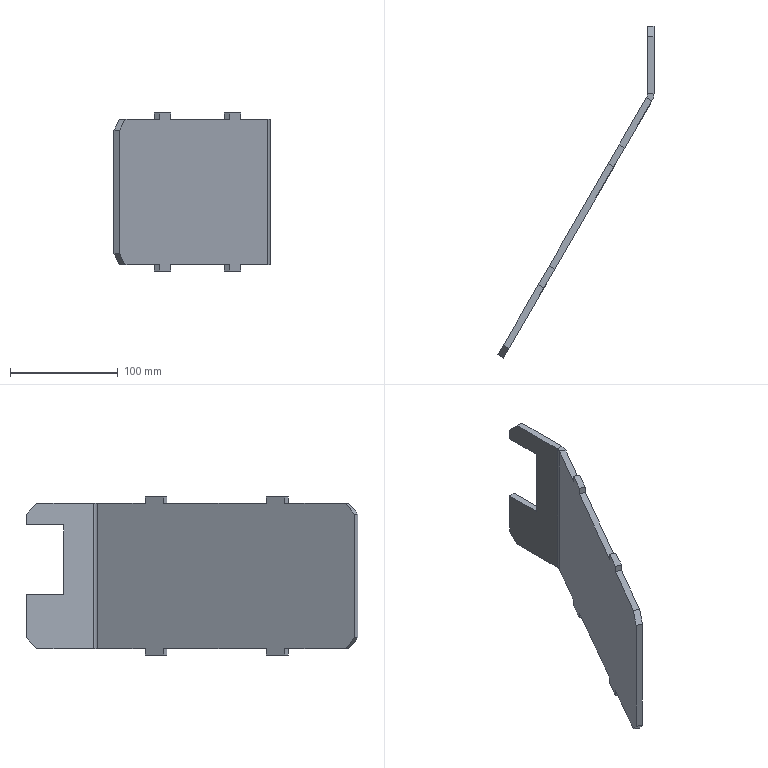Part | SolidWorks | features SMBaseFlange 2, Chamfer 1, Cut 1, FlatPattern 1, SheetMetal 1 | 1 solid | 38 faces | box 145.088 x 308.559 x 147 mm | volume 266913 mm3 | plane 36 | cylinder 2 | commonest cylinder face diameters 16 x1 28 x1
STEP:
#1=CARTESIAN_POINT('',(102.5,85.253,135.));
#2=VERTEX_POINT('',#1);
#3=CARTESIAN_POINT('',(157.5,180.516,135.));
#4=VERTEX_POINT('',#3);
#5=CARTESIAN_POINT('',(55.,2.981,135.));
#6=DIRECTION('',(0.5,0.866,0.));
#7=VECTOR('',#6,1000.);
#8=LINE('',#5,#7);
#9=EDGE_CURVE('',#2,#4,#8,.T.);
#10=ORIENTED_EDGE('',*,*,#9,.F.);
#11=CARTESIAN_POINT('',(107.696,82.253,135.));
#12=VERTEX_POINT('',#11);
#13=CARTESIAN_POINT('',(107.696,82.253,135.));
#14=DIRECTION('',(-0.866,0.5,0.));
#15=VECTOR('',#14,1000.);
#16=LINE('',#13,#15);
#17=EDGE_CURVE('',#12,#2,#16,.T.);
#18=ORIENTED_EDGE('',*,*,#17,.F.);
#19=CARTESIAN_POINT('',(162.696,177.516,135.));
#20=VERTEX_POINT('',#19);
#21=CARTESIAN_POINT('',(60.196,-0.01924,135.));
#22=DIRECTION('',(0.5,0.866,0.));
#23=VECTOR('',#22,1000.);
#24=LINE('',#21,#23);
#25=EDGE_CURVE('',#12,#20,#24,.T.);
#26=ORIENTED_EDGE('',*,*,#25,.T.);
#27=CARTESIAN_POINT('',(162.696,177.516,135.));
#28=DIRECTION('',(-0.866,0.5,0.));
#29=VECTOR('',#28,1000.);
#30=LINE('',#27,#29);
#31=EDGE_CURVE('',#20,#4,#30,.T.);
#32=ORIENTED_EDGE('',*,*,#31,.T.);
#33=EDGE_LOOP('',(#10,#18,#26,#32));
#34=FACE_OUTER_BOUND('',#33,.T.);
#35=CARTESIAN_POINT('',(186.088,246.032,135.));
#36=DIRECTION('',(0.,0.,-1.));
#37=DIRECTION('',(-1.,0.,0.));
#38=AXIS2_PLACEMENT_3D('',#35,#36,#37);
#39=PLANE('',#38);
#40=ADVANCED_FACE('',(#34),#39,.F.);
#41=CARTESIAN_POINT('',(167.5,197.836,135.));
#42=VERTEX_POINT('',#41);
#43=CARTESIAN_POINT('',(193.016,242.032,135.));
#44=VERTEX_POINT('',#43);
#45=CARTESIAN_POINT('',(55.,2.981,135.));
#46=DIRECTION('',(0.5,0.866,0.));
#47=VECTOR('',#46,1000.);
#48=LINE('',#45,#47);
#49=EDGE_CURVE('',#42,#44,#48,.T.);
#50=ORIENTED_EDGE('',*,*,#49,.F.);
#51=CARTESIAN_POINT('',(172.696,194.836,135.));
#52=VERTEX_POINT('',#51);
#53=CARTESIAN_POINT('',(172.696,194.836,135.));
#54=DIRECTION('',(-0.866,0.5,0.));
#55=VECTOR('',#54,1000.);
#56=LINE('',#53,#55);
#57=EDGE_CURVE('',#52,#42,#56,.T.);
#58=ORIENTED_EDGE('',*,*,#57,.F.);
#59=CARTESIAN_POINT('',(198.213,239.032,135.));
#60=VERTEX_POINT('',#59);
#61=CARTESIAN_POINT('',(60.196,-0.01924,135.));
#62=DIRECTION('',(0.5,0.866,0.));
#63=VECTOR('',#62,1000.);
#64=LINE('',#61,#63);
#65=EDGE_CURVE('',#52,#60,#64,.T.);
#66=ORIENTED_EDGE('',*,*,#65,.T.);
#67=CARTESIAN_POINT('',(198.213,239.032,135.));
#68=DIRECTION('',(-0.866,0.5,0.));
#69=VECTOR('',#68,1000.);
#70=LINE('',#67,#69);
#71=EDGE_CURVE('',#60,#44,#70,.T.);
#72=ORIENTED_EDGE('',*,*,#71,.T.);
#73=EDGE_LOOP('',(#50,#58,#66,#72));
#74=FACE_OUTER_BOUND('',#73,.T.);
#75=CARTESIAN_POINT('',(186.088,246.032,135.));
#76=DIRECTION('',(0.,0.,-1.));
#77=DIRECTION('',(-1.,0.,0.));
#78=AXIS2_PLACEMENT_3D('',#75,#76,#77);
#79=PLANE('',#78);
#80=ADVANCED_FACE('',(#74),#79,.F.);
#81=CARTESIAN_POINT('',(162.696,177.516,0.));
#82=VERTEX_POINT('',#81);
#83=CARTESIAN_POINT('',(157.5,180.516,0.));
#84=VERTEX_POINT('',#83);
#85=CARTESIAN_POINT('',(162.696,177.516,0.));
#86=DIRECTION('',(-0.866,0.5,0.));
#87=VECTOR('',#86,1000.);
#88=LINE('',#85,#87);
#89=EDGE_CURVE('',#82,#84,#88,.T.);
#90=ORIENTED_EDGE('',*,*,#89,.F.);
#91=CARTESIAN_POINT('',(107.696,82.253,0.));
#92=VERTEX_POINT('',#91);
#93=CARTESIAN_POINT('',(60.196,-0.01924,0.));
#94=DIRECTION('',(0.5,0.866,0.));
#95=VECTOR('',#94,1000.);
#96=LINE('',#93,#95);
#97=EDGE_CURVE('',#92,#82,#96,.T.);
#98=ORIENTED_EDGE('',*,*,#97,.F.);
#99=CARTESIAN_POINT('',(102.5,85.253,0.));
#100=VERTEX_POINT('',#99);
#101=CARTESIAN_POINT('',(107.696,82.253,0.));
#102=DIRECTION('',(-0.866,0.5,0.));
#103=VECTOR('',#102,1000.);
#104=LINE('',#101,#103);
#105=EDGE_CURVE('',#92,#100,#104,.T.);
#106=ORIENTED_EDGE('',*,*,#105,.T.);
#107=CARTESIAN_POINT('',(55.,2.981,0.));
#108=DIRECTION('',(0.5,0.866,0.));
#109=VECTOR('',#108,1000.);
#110=LINE('',#107,#109);
#111=EDGE_CURVE('',#100,#84,#110,.T.);
#112=ORIENTED_EDGE('',*,*,#111,.T.);
#113=EDGE_LOOP('',(#90,#98,#106,#112));
#114=FACE_OUTER_BOUND('',#113,.T.);
#115=CARTESIAN_POINT('',(200.088,246.032,0.));
#116=DIRECTION('',(0.,0.,-1.));
#117=DIRECTION('',(-1.,0.,0.));
#118=AXIS2_PLACEMENT_3D('',#115,#116,#117);
#119=PLANE('',#118);
#120=ADVANCED_FACE('',(#114),#119,.T.);
#121=CARTESIAN_POINT('',(65.196,8.641,0.));
#122=VERTEX_POINT('',#121);
#123=CARTESIAN_POINT('',(97.696,64.933,0.));
#124=VERTEX_POINT('',#123);
#125=CARTESIAN_POINT('',(60.196,-0.01924,0.));
#126=DIRECTION('',(0.5,0.866,0.));
#127=VECTOR('',#126,1000.);
#128=LINE('',#125,#127);
#129=EDGE_CURVE('',#122,#124,#128,.T.);
#130=ORIENTED_EDGE('',*,*,#129,.F.);
#131=CARTESIAN_POINT('',(60.,11.641,0.));
#132=VERTEX_POINT('',#131);
#133=CARTESIAN_POINT('',(63.572,9.579,0.));
#134=DIRECTION('',(-0.866,0.5,0.));
#135=VECTOR('',#134,1000.);
#136=LINE('',#133,#135);
#137=EDGE_CURVE('',#122,#132,#136,.T.);
#138=ORIENTED_EDGE('',*,*,#137,.T.);
#139=CARTESIAN_POINT('',(92.5,67.933,0.));
#140=VERTEX_POINT('',#139);
#141=CARTESIAN_POINT('',(55.,2.981,0.));
#142=DIRECTION('',(0.5,0.866,0.));
#143=VECTOR('',#142,1000.);
#144=LINE('',#141,#143);
#145=EDGE_CURVE('',#132,#140,#144,.T.);
#146=ORIENTED_EDGE('',*,*,#145,.T.);
#147=CARTESIAN_POINT('',(97.696,64.933,0.));
#148=DIRECTION('',(-0.866,0.5,0.));
#149=VECTOR('',#148,1000.);
#150=LINE('',#147,#149);
#151=EDGE_CURVE('',#124,#140,#150,.T.);
#152=ORIENTED_EDGE('',*,*,#151,.F.);
#153=EDGE_LOOP('',(#130,#138,#146,#152));
#154=FACE_OUTER_BOUND('',#153,.T.);
#155=CARTESIAN_POINT('',(200.088,246.032,0.));
#156=DIRECTION('',(0.,0.,-1.));
#157=DIRECTION('',(-1.,0.,0.));
#158=AXIS2_PLACEMENT_3D('',#155,#156,#157);
#159=PLANE('',#158);
#160=ADVANCED_FACE('',(#154),#159,.T.);
#161=CARTESIAN_POINT('',(200.088,308.54,125.));
#162=VERTEX_POINT('',#161);
#163=CARTESIAN_POINT('',(200.088,308.54,115.));
#164=VERTEX_POINT('',#163);
#165=CARTESIAN_POINT('',(200.088,308.54,135.));
#166=DIRECTION('',(0.,0.,-1.));
#167=VECTOR('',#166,1000.);
#168=LINE('',#165,#167);
#169=EDGE_CURVE('',#162,#164,#168,.T.);
#170=ORIENTED_EDGE('',*,*,#169,.F.);
#171=CARTESIAN_POINT('',(200.088,298.54,135.));
#172=VERTEX_POINT('',#171);
#173=CARTESIAN_POINT('',(200.088,308.54,125.));
#174=DIRECTION('',(0.,-0.7071,0.7071));
#175=VECTOR('',#174,1000.);
#176=LINE('',#173,#175);
#177=EDGE_CURVE('',#162,#172,#176,.T.);
#178=ORIENTED_EDGE('',*,*,#177,.T.);
#179=CARTESIAN_POINT('',(200.088,246.032,135.));
#180=VERTEX_POINT('',#179);
#181=CARTESIAN_POINT('',(200.088,243.889,135.));
#182=DIRECTION('',(0.,1.,0.));
#183=VECTOR('',#182,1000.);
#184=LINE('',#181,#183);
#185=EDGE_CURVE('',#180,#172,#184,.T.);
#186=ORIENTED_EDGE('',*,*,#185,.F.);
#187=CARTESIAN_POINT('',(200.088,246.032,0.));
#188=VERTEX_POINT('',#187);
#189=CARTESIAN_POINT('',(200.088,246.032,135.));
#190=DIRECTION('',(0.,0.,-1.));
#191=VECTOR('',#190,1000.);
#192=LINE('',#189,#191);
#193=EDGE_CURVE('',#180,#188,#192,.T.);
#194=ORIENTED_EDGE('',*,*,#193,.T.);
#195=CARTESIAN_POINT('',(200.088,298.54,0.));
#196=VERTEX_POINT('',#195);
#197=CARTESIAN_POINT('',(200.088,243.889,0.));
#198=DIRECTION('',(0.,1.,0.));
#199=VECTOR('',#198,1000.);
#200=LINE('',#197,#199);
#201=EDGE_CURVE('',#188,#196,#200,.T.);
#202=ORIENTED_EDGE('',*,*,#201,.T.);
#203=CARTESIAN_POINT('',(200.088,308.54,10.));
#204=VERTEX_POINT('',#203);
#205=CARTESIAN_POINT('',(200.088,298.54,0.));
#206=DIRECTION('',(0.,0.7071,0.7071));
#207=VECTOR('',#206,1000.);
#208=LINE('',#205,#207);
#209=EDGE_CURVE('',#196,#204,#208,.T.);
#210=ORIENTED_EDGE('',*,*,#209,.T.);
#211=CARTESIAN_POINT('',(200.088,308.54,50.));
#212=VERTEX_POINT('',#211);
#213=CARTESIAN_POINT('',(200.088,308.54,135.));
#214=DIRECTION('',(0.,0.,-1.));
#215=VECTOR('',#214,1000.);
#216=LINE('',#213,#215);
#217=EDGE_CURVE('',#212,#204,#216,.T.);
#218=ORIENTED_EDGE('',*,*,#217,.F.);
#219=CARTESIAN_POINT('',(200.088,273.54,50.));
#220=VERTEX_POINT('',#219);
#221=CARTESIAN_POINT('',(200.088,243.889,50.));
#222=DIRECTION('',(0.,1.,0.));
#223=VECTOR('',#222,1000.);
#224=LINE('',#221,#223);
#225=EDGE_CURVE('',#220,#212,#224,.T.);
#226=ORIENTED_EDGE('',*,*,#225,.F.);
#227=CARTESIAN_POINT('',(200.088,273.54,115.));
#228=VERTEX_POINT('',#227);
#229=CARTESIAN_POINT('',(200.088,273.54,135.));
#230=DIRECTION('',(0.,0.,-1.));
#231=VECTOR('',#230,1000.);
#232=LINE('',#229,#231);
#233=EDGE_CURVE('',#228,#220,#232,.T.);
#234=ORIENTED_EDGE('',*,*,#233,.F.);
#235=CARTESIAN_POINT('',(200.088,243.889,115.));
#236=DIRECTION('',(0.,-1.,0.));
#237=VECTOR('',#236,1000.);
#238=LINE('',#235,#237);
#239=EDGE_CURVE('',#164,#228,#238,.T.);
#240=ORIENTED_EDGE('',*,*,#239,.F.);
#241=EDGE_LOOP('',(#170,#178,#186,#194,#202,#210,#218,#226,#234,#240));
#242=FACE_OUTER_BOUND('',#241,.T.);
#243=CARTESIAN_POINT('',(200.088,243.889,135.));
#244=DIRECTION('',(-1.,0.,0.));
#245=DIRECTION('',(0.,-1.,0.));
#246=AXIS2_PLACEMENT_3D('',#243,#244,#245);
#247=PLANE('',#246);
#248=ADVANCED_FACE('',(#242),#247,.F.);
#249=ORIENTED_EDGE('',*,*,#217,.T.);
#250=CARTESIAN_POINT('',(194.088,308.54,10.));
#251=VERTEX_POINT('',#250);
#252=CARTESIAN_POINT('',(194.088,308.54,10.));
#253=DIRECTION('',(-1.,0.,0.));
#254=VECTOR('',#253,1000.);
#255=LINE('',#252,#254);
#256=EDGE_CURVE('',#204,#251,#255,.T.);
#257=ORIENTED_EDGE('',*,*,#256,.T.);
#258=CARTESIAN_POINT('',(194.088,308.54,50.));
#259=VERTEX_POINT('',#258);
#260=CARTESIAN_POINT('',(194.088,308.54,135.));
#261=DIRECTION('',(0.,0.,-1.));
#262=VECTOR('',#261,1000.);
#263=LINE('',#260,#262);
#264=EDGE_CURVE('',#259,#251,#263,.T.);
#265=ORIENTED_EDGE('',*,*,#264,.F.);
#266=CARTESIAN_POINT('',(200.088,308.54,50.));
#267=DIRECTION('',(-1.,0.,0.));
#268=VECTOR('',#267,1000.);
#269=LINE('',#266,#268);
#270=EDGE_CURVE('',#212,#259,#269,.T.);
#271=ORIENTED_EDGE('',*,*,#270,.F.);
#272=EDGE_LOOP('',(#249,#257,#265,#271));
#273=FACE_OUTER_BOUND('',#272,.T.);
#274=CARTESIAN_POINT('',(194.088,308.54,135.));
#275=DIRECTION('',(0.,1.,0.));
#276=DIRECTION('',(0.,0.,1.));
#277=AXIS2_PLACEMENT_3D('',#274,#275,#276);
#278=PLANE('',#277);
#279=ADVANCED_FACE('',(#273),#278,.T.);
#280=CARTESIAN_POINT('',(194.088,308.54,125.));
#281=VERTEX_POINT('',#280);
#282=CARTESIAN_POINT('',(194.088,308.54,115.));
#283=VERTEX_POINT('',#282);
#284=CARTESIAN_POINT('',(194.088,308.54,135.));
#285=DIRECTION('',(0.,0.,-1.));
#286=VECTOR('',#285,1000.);
#287=LINE('',#284,#286);
#288=EDGE_CURVE('',#281,#283,#287,.T.);
#289=ORIENTED_EDGE('',*,*,#288,.F.);
#290=CARTESIAN_POINT('',(194.088,308.54,125.));
#291=DIRECTION('',(1.,0.,0.));
#292=VECTOR('',#291,1000.);
#293=LINE('',#290,#292);
#294=EDGE_CURVE('',#281,#162,#293,.T.);
#295=ORIENTED_EDGE('',*,*,#294,.T.);
#296=ORIENTED_EDGE('',*,*,#169,.T.);
#297=CARTESIAN_POINT('',(200.088,308.54,115.));
#298=DIRECTION('',(-1.,0.,0.));
#299=VECTOR('',#298,1000.);
#300=LINE('',#297,#299);
#301=EDGE_CURVE('',#164,#283,#300,.T.);
#302=ORIENTED_EDGE('',*,*,#301,.T.);
#303=EDGE_LOOP('',(#289,#295,#296,#302));
#304=FACE_OUTER_BOUND('',#303,.T.);
#305=CARTESIAN_POINT('',(194.088,308.54,135.));
#306=DIRECTION('',(0.,1.,0.));
#307=DIRECTION('',(0.,0.,1.));
#308=AXIS2_PLACEMENT_3D('',#305,#306,#307);
#309=PLANE('',#308);
#310=ADVANCED_FACE('',(#304),#309,.T.);
#311=CARTESIAN_POINT('',(194.088,246.032,135.));
#312=VERTEX_POINT('',#311);
#313=CARTESIAN_POINT('',(194.088,298.54,135.));
#314=VERTEX_POINT('',#313);
#315=CARTESIAN_POINT('',(194.088,243.889,135.));
#316=DIRECTION('',(0.,1.,0.));
#317=VECTOR('',#316,1000.);
#318=LINE('',#315,#317);
#319=EDGE_CURVE('',#312,#314,#318,.T.);
#320=ORIENTED_EDGE('',*,*,#319,.T.);
#321=CARTESIAN_POINT('',(194.088,271.214,162.326));
#322=DIRECTION('',(0.,0.7071,-0.7071));
#323=VECTOR('',#322,1000.);
#324=LINE('',#321,#323);
#325=EDGE_CURVE('',#314,#281,#324,.T.);
#326=ORIENTED_EDGE('',*,*,#325,.T.);
#327=ORIENTED_EDGE('',*,*,#288,.T.);
#328=CARTESIAN_POINT('',(194.088,273.54,115.));
#329=VERTEX_POINT('',#328);
#330=CARTESIAN_POINT('',(194.088,308.54,115.));
#331=DIRECTION('',(0.,-1.,0.));
#332=VECTOR('',#331,1000.);
#333=LINE('',#330,#332);
#334=EDGE_CURVE('',#283,#329,#333,.T.);
#335=ORIENTED_EDGE('',*,*,#334,.T.);
#336=CARTESIAN_POINT('',(194.088,273.54,50.));
#337=VERTEX_POINT('',#336);
#338=CARTESIAN_POINT('',(194.088,273.54,50.));
#339=DIRECTION('',(0.,0.,-1.));
#340=VECTOR('',#339,1000.);
#341=LINE('',#338,#340);
#342=EDGE_CURVE('',#329,#337,#341,.T.);
#343=ORIENTED_EDGE('',*,*,#342,.T.);
#344=CARTESIAN_POINT('',(194.088,308.54,50.));
#345=DIRECTION('',(0.,1.,0.));
#346=VECTOR('',#345,1000.);
#347=LINE('',#344,#346);
#348=EDGE_CURVE('',#337,#259,#347,.T.);
#349=ORIENTED_EDGE('',*,*,#348,.T.);
#350=ORIENTED_EDGE('',*,*,#264,.T.);
#351=CARTESIAN_POINT('',(194.088,298.54,0.));
#352=VERTEX_POINT('',#351);
#353=CARTESIAN_POINT('',(194.088,338.714,40.174));
#354=DIRECTION('',(0.,-0.7071,-0.7071));
#355=VECTOR('',#354,1000.);
#356=LINE('',#353,#355);
#357=EDGE_CURVE('',#251,#352,#356,.T.);
#358=ORIENTED_EDGE('',*,*,#357,.T.);
#359=CARTESIAN_POINT('',(194.088,246.032,0.));
#360=VERTEX_POINT('',#359);
#361=CARTESIAN_POINT('',(194.088,243.889,0.));
#362=DIRECTION('',(0.,1.,0.));
#363=VECTOR('',#362,1000.);
#364=LINE('',#361,#363);
#365=EDGE_CURVE('',#360,#352,#364,.T.);
#366=ORIENTED_EDGE('',*,*,#365,.F.);
#367=CARTESIAN_POINT('',(194.088,246.032,135.));
#368=DIRECTION('',(0.,0.,-1.));
#369=VECTOR('',#368,1000.);
#370=LINE('',#367,#369);
#371=EDGE_CURVE('',#312,#360,#370,.T.);
#372=ORIENTED_EDGE('',*,*,#371,.F.);
#373=EDGE_LOOP('',(#320,#326,#327,#335,#343,#349,#350,#358,#366,#372));
#374=FACE_OUTER_BOUND('',#373,.T.);
#375=CARTESIAN_POINT('',(194.088,243.889,135.));
#376=DIRECTION('',(-1.,0.,0.));
#377=DIRECTION('',(0.,-1.,0.));
#378=AXIS2_PLACEMENT_3D('',#375,#376,#377);
#379=PLANE('',#378);
#380=ADVANCED_FACE('',(#374),#379,.T.);
#381=CARTESIAN_POINT('',(194.088,246.032,135.));
#382=DIRECTION('',(1.,0.,0.));
#383=VECTOR('',#382,1000.);
#384=LINE('',#381,#383);
#385=EDGE_CURVE('',#312,#180,#384,.T.);
#386=ORIENTED_EDGE('',*,*,#385,.F.);
#387=CARTESIAN_POINT('',(186.088,246.032,135.));
#388=DIRECTION('',(0.,0.,1.));
#389=DIRECTION('',(-1.,0.,0.));
#390=AXIS2_PLACEMENT_3D('',#387,#388,#389);
#391=CIRCLE('',#390,8.);
#392=EDGE_CURVE('',#44,#312,#391,.T.);
#393=ORIENTED_EDGE('',*,*,#392,.F.);
#394=ORIENTED_EDGE('',*,*,#71,.F.);
#395=CARTESIAN_POINT('',(186.088,246.032,135.));
#396=DIRECTION('',(0.,0.,1.));
#397=DIRECTION('',(1.,0.,0.));
#398=AXIS2_PLACEMENT_3D('',#395,#396,#397);
#399=CIRCLE('',#398,14.);
#400=EDGE_CURVE('',#60,#180,#399,.T.);
#401=ORIENTED_EDGE('',*,*,#400,.T.);
#402=EDGE_LOOP('',(#386,#393,#394,#401));
#403=FACE_OUTER_BOUND('',#402,.T.);
#404=CARTESIAN_POINT('',(194.088,246.032,135.));
#405=DIRECTION('',(0.,0.,1.));
#406=DIRECTION('',(1.,0.,0.));
#407=AXIS2_PLACEMENT_3D('',#404,#405,#406);
#408=PLANE('',#407);
#409=ADVANCED_FACE('',(#403),#408,.T.);
#410=ORIENTED_EDGE('',*,*,#185,.T.);
#411=CARTESIAN_POINT('',(198.213,298.54,135.));
#412=DIRECTION('',(-1.,0.,0.));
#413=VECTOR('',#412,1000.);
#414=LINE('',#411,#413);
#415=EDGE_CURVE('',#172,#314,#414,.T.);
#416=ORIENTED_EDGE('',*,*,#415,.T.);
#417=ORIENTED_EDGE('',*,*,#319,.F.);
#418=ORIENTED_EDGE('',*,*,#385,.T.);
#419=EDGE_LOOP('',(#410,#416,#417,#418));
#420=FACE_OUTER_BOUND('',#419,.T.);
#421=CARTESIAN_POINT('',(198.213,239.032,135.));
#422=DIRECTION('',(0.,0.,1.));
#423=DIRECTION('',(1.,0.,0.));
#424=AXIS2_PLACEMENT_3D('',#421,#422,#423);
#425=PLANE('',#424);
#426=ADVANCED_FACE('',(#420),#425,.T.);
#427=CARTESIAN_POINT('',(193.016,242.032,0.));
#428=VERTEX_POINT('',#427);
#429=CARTESIAN_POINT('',(198.213,239.032,0.));
#430=VERTEX_POINT('',#429);
#431=CARTESIAN_POINT('',(193.016,242.032,0.));
#432=DIRECTION('',(0.866,-0.5,0.));
#433=VECTOR('',#432,1000.);
#434=LINE('',#431,#433);
#435=EDGE_CURVE('',#428,#430,#434,.T.);
#436=ORIENTED_EDGE('',*,*,#435,.F.);
#437=CARTESIAN_POINT('',(186.088,246.032,0.));
#438=DIRECTION('',(0.,0.,1.));
#439=DIRECTION('',(-1.,0.,0.));
#440=AXIS2_PLACEMENT_3D('',#437,#438,#439);
#441=CIRCLE('',#440,8.);
#442=EDGE_CURVE('',#428,#360,#441,.T.);
#443=ORIENTED_EDGE('',*,*,#442,.T.);
#444=CARTESIAN_POINT('',(200.088,246.032,0.));
#445=DIRECTION('',(-1.,0.,0.));
#446=VECTOR('',#445,1000.);
#447=LINE('',#444,#446);
#448=EDGE_CURVE('',#188,#360,#447,.T.);
#449=ORIENTED_EDGE('',*,*,#448,.F.);
#450=CARTESIAN_POINT('',(186.088,246.032,0.));
#451=DIRECTION('',(0.,0.,1.));
#452=DIRECTION('',(1.,0.,0.));
#453=AXIS2_PLACEMENT_3D('',#450,#451,#452);
#454=CIRCLE('',#453,14.);
#455=EDGE_CURVE('',#430,#188,#454,.T.);
#456=ORIENTED_EDGE('',*,*,#455,.F.);
#457=EDGE_LOOP('',(#436,#443,#449,#456));
#458=FACE_OUTER_BOUND('',#457,.T.);
#459=CARTESIAN_POINT('',(193.016,242.032,0.));
#460=DIRECTION('',(0.,0.,-1.));
#461=DIRECTION('',(-1.,0.,0.));
#462=AXIS2_PLACEMENT_3D('',#459,#460,#461);
#463=PLANE('',#462);
#464=ADVANCED_FACE('',(#458),#463,.T.);
#465=CARTESIAN_POINT('',(172.696,194.836,0.));
#466=VERTEX_POINT('',#465);
#467=CARTESIAN_POINT('',(167.5,197.836,0.));
#468=VERTEX_POINT('',#467);
#469=CARTESIAN_POINT('',(172.696,194.836,0.));
#470=DIRECTION('',(-0.866,0.5,0.));
#471=VECTOR('',#470,1000.);
#472=LINE('',#469,#471);
#473=EDGE_CURVE('',#466,#468,#472,.T.);
#474=ORIENTED_EDGE('',*,*,#473,.T.);
#475=CARTESIAN_POINT('',(55.,2.981,0.));
#476=DIRECTION('',(0.5,0.866,0.));
#477=VECTOR('',#476,1000.);
#478=LINE('',#475,#477);
#479=EDGE_CURVE('',#468,#428,#478,.T.);
#480=ORIENTED_EDGE('',*,*,#479,.T.);
#481=ORIENTED_EDGE('',*,*,#435,.T.);
#482=CARTESIAN_POINT('',(60.196,-0.01924,0.));
#483=DIRECTION('',(0.5,0.866,0.));
#484=VECTOR('',#483,1000.);
#485=LINE('',#482,#484);
#486=EDGE_CURVE('',#466,#430,#485,.T.);
#487=ORIENTED_EDGE('',*,*,#486,.F.);
#488=EDGE_LOOP('',(#474,#480,#481,#487));
#489=FACE_OUTER_BOUND('',#488,.T.);
#490=CARTESIAN_POINT('',(200.088,246.032,0.));
#491=DIRECTION('',(0.,0.,-1.));
#492=DIRECTION('',(-1.,0.,0.));
#493=AXIS2_PLACEMENT_3D('',#490,#491,#492);
#494=PLANE('',#493);
#495=ADVANCED_FACE('',(#489),#494,.T.);
#496=ORIENTED_EDGE('',*,*,#442,.F.);
#497=CARTESIAN_POINT('',(193.016,242.032,135.));
#498=DIRECTION('',(0.,0.,-1.));
#499=VECTOR('',#498,1000.);
#500=LINE('',#497,#499);
#501=EDGE_CURVE('',#44,#428,#500,.T.);
#502=ORIENTED_EDGE('',*,*,#501,.F.);
#503=ORIENTED_EDGE('',*,*,#392,.T.);
#504=ORIENTED_EDGE('',*,*,#371,.T.);
#505=EDGE_LOOP('',(#496,#502,#503,#504));
#506=FACE_OUTER_BOUND('',#505,.T.);
#507=CARTESIAN_POINT('',(186.088,246.032,135.));
#508=DIRECTION('',(0.,0.,-1.));
#509=DIRECTION('',(-1.,0.,0.));
#510=AXIS2_PLACEMENT_3D('',#507,#508,#509);
#511=CYLINDRICAL_SURFACE('',#510,8.);
#512=ADVANCED_FACE('',(#506),#511,.F.);
#513=ORIENTED_EDGE('',*,*,#145,.F.);
#514=CARTESIAN_POINT('',(55.,2.981,10.));
#515=VERTEX_POINT('',#514);
#516=CARTESIAN_POINT('',(23.75,-51.146,72.5));
#517=DIRECTION('',(-0.3536,-0.6124,0.7071));
#518=VECTOR('',#517,1000.);
#519=LINE('',#516,#518);
#520=EDGE_CURVE('',#132,#515,#519,.T.);
#521=ORIENTED_EDGE('',*,*,#520,.T.);
#522=CARTESIAN_POINT('',(55.,2.981,125.));
#523=VERTEX_POINT('',#522);
#524=CARTESIAN_POINT('',(55.,2.981,135.));
#525=DIRECTION('',(0.,0.,-1.));
#526=VECTOR('',#525,1000.);
#527=LINE('',#524,#526);
#528=EDGE_CURVE('',#523,#515,#527,.T.);
#529=ORIENTED_EDGE('',*,*,#528,.F.);
#530=CARTESIAN_POINT('',(60.,11.641,135.));
#531=VERTEX_POINT('',#530);
#532=CARTESIAN_POINT('',(57.5,7.311,130.));
#533=DIRECTION('',(0.3536,0.6124,0.7071));
#534=VECTOR('',#533,1000.);
#535=LINE('',#532,#534);
#536=EDGE_CURVE('',#523,#531,#535,.T.);
#537=ORIENTED_EDGE('',*,*,#536,.T.);
#538=CARTESIAN_POINT('',(92.5,67.933,135.));
#539=VERTEX_POINT('',#538);
#540=CARTESIAN_POINT('',(55.,2.981,135.));
#541=DIRECTION('',(0.5,0.866,0.));
#542=VECTOR('',#541,1000.);
#543=LINE('',#540,#542);
#544=EDGE_CURVE('',#531,#539,#543,.T.);
#545=ORIENTED_EDGE('',*,*,#544,.T.);
#546=CARTESIAN_POINT('',(92.5,67.933,141.));
#547=VERTEX_POINT('',#546);
#548=CARTESIAN_POINT('',(92.5,67.933,135.));
#549=DIRECTION('',(0.,0.,1.));
#550=VECTOR('',#549,1000.);
#551=LINE('',#548,#550);
#552=EDGE_CURVE('',#539,#547,#551,.T.);
#553=ORIENTED_EDGE('',*,*,#552,.T.);
#554=CARTESIAN_POINT('',(102.5,85.253,141.));
#555=VERTEX_POINT('',#554);
#556=CARTESIAN_POINT('',(92.5,67.933,141.));
#557=DIRECTION('',(0.5,0.866,0.));
#558=VECTOR('',#557,1000.);
#559=LINE('',#556,#558);
#560=EDGE_CURVE('',#547,#555,#559,.T.);
#561=ORIENTED_EDGE('',*,*,#560,.T.);
#562=CARTESIAN_POINT('',(102.5,85.253,141.));
#563=DIRECTION('',(0.,0.,-1.));
#564=VECTOR('',#563,1000.);
#565=LINE('',#562,#564);
#566=EDGE_CURVE('',#555,#2,#565,.T.);
#567=ORIENTED_EDGE('',*,*,#566,.T.);
#568=ORIENTED_EDGE('',*,*,#9,.T.);
#569=CARTESIAN_POINT('',(157.5,180.516,141.));
#570=VERTEX_POINT('',#569);
#571=CARTESIAN_POINT('',(157.5,180.516,135.));
#572=DIRECTION('',(0.,0.,1.));
#573=VECTOR('',#572,1000.);
#574=LINE('',#571,#573);
#575=EDGE_CURVE('',#4,#570,#574,.T.);
#576=ORIENTED_EDGE('',*,*,#575,.T.);
#577=CARTESIAN_POINT('',(167.5,197.836,141.));
#578=VERTEX_POINT('',#577);
#579=CARTESIAN_POINT('',(157.5,180.516,141.));
#580=DIRECTION('',(0.5,0.866,0.));
#581=VECTOR('',#580,1000.);
#582=LINE('',#579,#581);
#583=EDGE_CURVE('',#570,#578,#582,.T.);
#584=ORIENTED_EDGE('',*,*,#583,.T.);
#585=CARTESIAN_POINT('',(167.5,197.836,141.));
#586=DIRECTION('',(0.,0.,-1.));
#587=VECTOR('',#586,1000.);
#588=LINE('',#585,#587);
#589=EDGE_CURVE('',#578,#42,#588,.T.);
#590=ORIENTED_EDGE('',*,*,#589,.T.);
#591=ORIENTED_EDGE('',*,*,#49,.T.);
#592=ORIENTED_EDGE('',*,*,#501,.T.);
#593=ORIENTED_EDGE('',*,*,#479,.F.);
#594=CARTESIAN_POINT('',(167.5,197.836,-6.));
#595=VERTEX_POINT('',#594);
#596=CARTESIAN_POINT('',(167.5,197.836,-6.));
#597=DIRECTION('',(0.,0.,-1.));
#598=VECTOR('',#597,1000.);
#599=LINE('',#596,#598);
#600=EDGE_CURVE('',#468,#595,#599,.T.);
#601=ORIENTED_EDGE('',*,*,#600,.T.);
#602=CARTESIAN_POINT('',(157.5,180.516,-6.));
#603=VERTEX_POINT('',#602);
#604=CARTESIAN_POINT('',(157.5,180.516,-6.));
#605=DIRECTION('',(-0.5,-0.866,0.));
#606=VECTOR('',#605,1000.);
#607=LINE('',#604,#606);
#608=EDGE_CURVE('',#595,#603,#607,.T.);
#609=ORIENTED_EDGE('',*,*,#608,.T.);
#610=CARTESIAN_POINT('',(157.5,180.516,0.));
#611=DIRECTION('',(0.,0.,1.));
#612=VECTOR('',#611,1000.);
#613=LINE('',#610,#612);
#614=EDGE_CURVE('',#603,#84,#613,.T.);
#615=ORIENTED_EDGE('',*,*,#614,.T.);
#616=ORIENTED_EDGE('',*,*,#111,.F.);
#617=CARTESIAN_POINT('',(102.5,85.253,-6.));
#618=VERTEX_POINT('',#617);
#619=CARTESIAN_POINT('',(102.5,85.253,-6.));
#620=DIRECTION('',(0.,0.,-1.));
#621=VECTOR('',#620,1000.);
#622=LINE('',#619,#621);
#623=EDGE_CURVE('',#100,#618,#622,.T.);
#624=ORIENTED_EDGE('',*,*,#623,.T.);
#625=CARTESIAN_POINT('',(92.5,67.933,-6.));
#626=VERTEX_POINT('',#625);
#627=CARTESIAN_POINT('',(92.5,67.933,-6.));
#628=DIRECTION('',(-0.5,-0.866,0.));
#629=VECTOR('',#628,1000.);
#630=LINE('',#627,#629);
#631=EDGE_CURVE('',#618,#626,#630,.T.);
#632=ORIENTED_EDGE('',*,*,#631,.T.);
#633=CARTESIAN_POINT('',(92.5,67.933,0.));
#634=DIRECTION('',(0.,0.,1.));
#635=VECTOR('',#634,1000.);
#636=LINE('',#633,#635);
#637=EDGE_CURVE('',#626,#140,#636,.T.);
#638=ORIENTED_EDGE('',*,*,#637,.T.);
#639=EDGE_LOOP('',(#513,#521,#529,#537,#545,#553,#561,#567,#568,#576,#584,#590,#591,#592,#593,#601,#609,#615,#616,#624,#632,#638));
#640=FACE_OUTER_BOUND('',#639,.T.);
#641=CARTESIAN_POINT('',(55.,2.981,135.));
#642=DIRECTION('',(-0.866,0.5,0.));
#643=DIRECTION('',(-0.5,-0.866,0.));
#644=AXIS2_PLACEMENT_3D('',#641,#642,#643);
#645=PLANE('',#644);
#646=ADVANCED_FACE('',(#640),#645,.T.);
#647=ORIENTED_EDGE('',*,*,#528,.T.);
#648=CARTESIAN_POINT('',(60.196,-0.01924,10.));
#649=VERTEX_POINT('',#648);
#650=CARTESIAN_POINT('',(60.196,-0.01924,10.));
#651=DIRECTION('',(0.866,-0.5,0.));
#652=VECTOR('',#651,1000.);
#653=LINE('',#650,#652);
#654=EDGE_CURVE('',#515,#649,#653,.T.);
#655=ORIENTED_EDGE('',*,*,#654,.T.);
#656=CARTESIAN_POINT('',(60.196,-0.01924,125.));
#657=VERTEX_POINT('',#656);
#658=CARTESIAN_POINT('',(60.196,-0.01924,135.));
#659=DIRECTION('',(0.,0.,-1.));
#660=VECTOR('',#659,1000.);
#661=LINE('',#658,#660);
#662=EDGE_CURVE('',#657,#649,#661,.T.);
#663=ORIENTED_EDGE('',*,*,#662,.F.);
#664=CARTESIAN_POINT('',(55.,2.981,125.));
#665=DIRECTION('',(-0.866,0.5,0.));
#666=VECTOR('',#665,1000.);
#667=LINE('',#664,#666);
#668=EDGE_CURVE('',#657,#523,#667,.T.);
#669=ORIENTED_EDGE('',*,*,#668,.T.);
#670=EDGE_LOOP('',(#647,#655,#663,#669));
#671=FACE_OUTER_BOUND('',#670,.T.);
#672=CARTESIAN_POINT('',(60.196,-0.01924,135.));
#673=DIRECTION('',(-0.5,-0.866,0.));
#674=DIRECTION('',(0.866,-0.5,0.));
#675=AXIS2_PLACEMENT_3D('',#672,#673,#674);
#676=PLANE('',#675);
#677=ADVANCED_FACE('',(#671),#676,.T.);
#678=ORIENTED_EDGE('',*,*,#662,.T.);
#679=CARTESIAN_POINT('',(65.196,8.641,0.));
#680=DIRECTION('',(0.3536,0.6124,-0.7071));
#681=VECTOR('',#680,1000.);
#682=LINE('',#679,#681);
#683=EDGE_CURVE('',#649,#122,#682,.T.);
#684=ORIENTED_EDGE('',*,*,#683,.T.);
#685=ORIENTED_EDGE('',*,*,#129,.T.);
#686=CARTESIAN_POINT('',(97.696,64.933,-6.));
#687=VERTEX_POINT('',#686);
#688=CARTESIAN_POINT('',(97.696,64.933,0.));
#689=DIRECTION('',(0.,0.,1.));
#690=VECTOR('',#689,1000.);
#691=LINE('',#688,#690);
#692=EDGE_CURVE('',#687,#124,#691,.T.);
#693=ORIENTED_EDGE('',*,*,#692,.F.);
#694=CARTESIAN_POINT('',(107.696,82.253,-6.));
#695=VERTEX_POINT('',#694);
#696=CARTESIAN_POINT('',(97.696,64.933,-6.));
#697=DIRECTION('',(-0.5,-0.866,0.));
#698=VECTOR('',#697,1000.);
#699=LINE('',#696,#698);
#700=EDGE_CURVE('',#695,#687,#699,.T.);
#701=ORIENTED_EDGE('',*,*,#700,.F.);
#702=CARTESIAN_POINT('',(107.696,82.253,-6.));
#703=DIRECTION('',(0.,0.,-1.));
#704=VECTOR('',#703,1000.);
#705=LINE('',#702,#704);
#706=EDGE_CURVE('',#92,#695,#705,.T.);
#707=ORIENTED_EDGE('',*,*,#706,.F.);
#708=ORIENTED_EDGE('',*,*,#97,.T.);
#709=CARTESIAN_POINT('',(162.696,177.516,-6.));
#710=VERTEX_POINT('',#709);
#711=CARTESIAN_POINT('',(162.696,177.516,0.));
#712=DIRECTION('',(0.,0.,1.));
#713=VECTOR('',#712,1000.);
#714=LINE('',#711,#713);
#715=EDGE_CURVE('',#710,#82,#714,.T.);
#716=ORIENTED_EDGE('',*,*,#715,.F.);
#717=CARTESIAN_POINT('',(172.696,194.836,-6.));
#718=VERTEX_POINT('',#717);
#719=CARTESIAN_POINT('',(162.696,177.516,-6.));
#720=DIRECTION('',(-0.5,-0.866,0.));
#721=VECTOR('',#720,1000.);
#722=LINE('',#719,#721);
#723=EDGE_CURVE('',#718,#710,#722,.T.);
#724=ORIENTED_EDGE('',*,*,#723,.F.);
#725=CARTESIAN_POINT('',(172.696,194.836,-6.));
#726=DIRECTION('',(0.,0.,-1.));
#727=VECTOR('',#726,1000.);
#728=LINE('',#725,#727);
#729=EDGE_CURVE('',#466,#718,#728,.T.);
#730=ORIENTED_EDGE('',*,*,#729,.F.);
#731=ORIENTED_EDGE('',*,*,#486,.T.);
#732=CARTESIAN_POINT('',(198.213,239.032,135.));
#733=DIRECTION('',(0.,0.,-1.));
#734=VECTOR('',#733,1000.);
#735=LINE('',#732,#734);
#736=EDGE_CURVE('',#60,#430,#735,.T.);
#737=ORIENTED_EDGE('',*,*,#736,.F.);
#738=ORIENTED_EDGE('',*,*,#65,.F.);
#739=CARTESIAN_POINT('',(172.696,194.836,141.));
#740=VERTEX_POINT('',#739);
#741=CARTESIAN_POINT('',(172.696,194.836,141.));
#742=DIRECTION('',(0.,0.,-1.));
#743=VECTOR('',#742,1000.);
#744=LINE('',#741,#743);
#745=EDGE_CURVE('',#740,#52,#744,.T.);
#746=ORIENTED_EDGE('',*,*,#745,.F.);
#747=CARTESIAN_POINT('',(162.696,177.516,141.));
#748=VERTEX_POINT('',#747);
#749=CARTESIAN_POINT('',(162.696,177.516,141.));
#750=DIRECTION('',(0.5,0.866,0.));
#751=VECTOR('',#750,1000.);
#752=LINE('',#749,#751);
#753=EDGE_CURVE('',#748,#740,#752,.T.);
#754=ORIENTED_EDGE('',*,*,#753,.F.);
#755=CARTESIAN_POINT('',(162.696,177.516,135.));
#756=DIRECTION('',(0.,0.,1.));
#757=VECTOR('',#756,1000.);
#758=LINE('',#755,#757);
#759=EDGE_CURVE('',#20,#748,#758,.T.);
#760=ORIENTED_EDGE('',*,*,#759,.F.);
#761=ORIENTED_EDGE('',*,*,#25,.F.);
#762=CARTESIAN_POINT('',(107.696,82.253,141.));
#763=VERTEX_POINT('',#762);
#764=CARTESIAN_POINT('',(107.696,82.253,141.));
#765=DIRECTION('',(0.,0.,-1.));
#766=VECTOR('',#765,1000.);
#767=LINE('',#764,#766);
#768=EDGE_CURVE('',#763,#12,#767,.T.);
#769=ORIENTED_EDGE('',*,*,#768,.F.);
#770=CARTESIAN_POINT('',(97.696,64.933,141.));
#771=VERTEX_POINT('',#770);
#772=CARTESIAN_POINT('',(97.696,64.933,141.));
#773=DIRECTION('',(0.5,0.866,0.));
#774=VECTOR('',#773,1000.);
#775=LINE('',#772,#774);
#776=EDGE_CURVE('',#771,#763,#775,.T.);
#777=ORIENTED_EDGE('',*,*,#776,.F.);
#778=CARTESIAN_POINT('',(97.696,64.933,135.));
#779=VERTEX_POINT('',#778);
#780=CARTESIAN_POINT('',(97.696,64.933,135.));
#781=DIRECTION('',(0.,0.,1.));
#782=VECTOR('',#781,1000.);
#783=LINE('',#780,#782);
#784=EDGE_CURVE('',#779,#771,#783,.T.);
#785=ORIENTED_EDGE('',*,*,#784,.F.);
#786=CARTESIAN_POINT('',(65.196,8.641,135.));
#787=VERTEX_POINT('',#786);
#788=CARTESIAN_POINT('',(60.196,-0.01924,135.));
#789=DIRECTION('',(0.5,0.866,0.));
#790=VECTOR('',#789,1000.);
#791=LINE('',#788,#790);
#792=EDGE_CURVE('',#787,#779,#791,.T.);
#793=ORIENTED_EDGE('',*,*,#792,.F.);
#794=CARTESIAN_POINT('',(60.196,-0.01924,125.));
#795=DIRECTION('',(-0.3536,-0.6124,-0.7071));
#796=VECTOR('',#795,1000.);
#797=LINE('',#794,#796);
#798=EDGE_CURVE('',#787,#657,#797,.T.);
#799=ORIENTED_EDGE('',*,*,#798,.T.);
#800=EDGE_LOOP('',(#678,#684,#685,#693,#701,#707,#708,#716,#724,#730,#731,#737,#738,#746,#754,#760,#761,#769,#777,#785,#793,#799));
#801=FACE_OUTER_BOUND('',#800,.T.);
#802=CARTESIAN_POINT('',(60.196,-0.01924,135.));
#803=DIRECTION('',(-0.866,0.5,0.));
#804=DIRECTION('',(-0.5,-0.866,0.));
#805=AXIS2_PLACEMENT_3D('',#802,#803,#804);
#806=PLANE('',#805);
#807=ADVANCED_FACE('',(#801),#806,.F.);
#808=ORIENTED_EDGE('',*,*,#455,.T.);
#809=ORIENTED_EDGE('',*,*,#193,.F.);
#810=ORIENTED_EDGE('',*,*,#400,.F.);
#811=ORIENTED_EDGE('',*,*,#736,.T.);
#812=EDGE_LOOP('',(#808,#809,#810,#811));
#813=FACE_OUTER_BOUND('',#812,.T.);
#814=CARTESIAN_POINT('',(186.088,246.032,135.));
#815=DIRECTION('',(0.,0.,-1.));
#816=DIRECTION('',(-1.,0.,0.));
#817=AXIS2_PLACEMENT_3D('',#814,#815,#816);
#818=CYLINDRICAL_SURFACE('',#817,14.);
#819=ADVANCED_FACE('',(#813),#818,.T.);
#820=ORIENTED_EDGE('',*,*,#544,.F.);
#821=CARTESIAN_POINT('',(65.196,8.641,135.));
#822=DIRECTION('',(0.866,-0.5,0.));
#823=VECTOR('',#822,1000.);
#824=LINE('',#821,#823);
#825=EDGE_CURVE('',#531,#787,#824,.T.);
#826=ORIENTED_EDGE('',*,*,#825,.T.);
#827=ORIENTED_EDGE('',*,*,#792,.T.);
#828=CARTESIAN_POINT('',(97.696,64.933,135.));
#829=DIRECTION('',(-0.866,0.5,0.));
#830=VECTOR('',#829,1000.);
#831=LINE('',#828,#830);
#832=EDGE_CURVE('',#779,#539,#831,.T.);
#833=ORIENTED_EDGE('',*,*,#832,.T.);
#834=EDGE_LOOP('',(#820,#826,#827,#833));
#835=FACE_OUTER_BOUND('',#834,.T.);
#836=CARTESIAN_POINT('',(186.088,246.032,135.));
#837=DIRECTION('',(0.,0.,-1.));
#838=DIRECTION('',(-1.,0.,0.));
#839=AXIS2_PLACEMENT_3D('',#836,#837,#838);
#840=PLANE('',#839);
#841=ADVANCED_FACE('',(#835),#840,.F.);
#842=ORIENTED_EDGE('',*,*,#365,.T.);
#843=CARTESIAN_POINT('',(186.088,298.54,0.));
#844=DIRECTION('',(1.,0.,0.));
#845=VECTOR('',#844,1000.);
#846=LINE('',#843,#845);
#847=EDGE_CURVE('',#352,#196,#846,.T.);
#848=ORIENTED_EDGE('',*,*,#847,.T.);
#849=ORIENTED_EDGE('',*,*,#201,.F.);
#850=ORIENTED_EDGE('',*,*,#448,.T.);
#851=EDGE_LOOP('',(#842,#848,#849,#850));
#852=FACE_OUTER_BOUND('',#851,.T.);
#853=CARTESIAN_POINT('',(186.088,246.032,0.));
#854=DIRECTION('',(0.,0.,-1.));
#855=DIRECTION('',(-1.,0.,0.));
#856=AXIS2_PLACEMENT_3D('',#853,#854,#855);
#857=PLANE('',#856);
#858=ADVANCED_FACE('',(#852),#857,.T.);
#859=ORIENTED_EDGE('',*,*,#233,.T.);
#860=CARTESIAN_POINT('',(200.088,273.54,50.));
#861=DIRECTION('',(-1.,0.,0.));
#862=VECTOR('',#861,1000.);
#863=LINE('',#860,#862);
#864=EDGE_CURVE('',#220,#337,#863,.T.);
#865=ORIENTED_EDGE('',*,*,#864,.T.);
#866=ORIENTED_EDGE('',*,*,#342,.F.);
#867=CARTESIAN_POINT('',(200.088,273.54,115.));
#868=DIRECTION('',(-1.,0.,0.));
#869=VECTOR('',#868,1000.);
#870=LINE('',#867,#869);
#871=EDGE_CURVE('',#228,#329,#870,.T.);
#872=ORIENTED_EDGE('',*,*,#871,.F.);
#873=EDGE_LOOP('',(#859,#865,#866,#872));
#874=FACE_OUTER_BOUND('',#873,.T.);
#875=CARTESIAN_POINT('',(200.088,273.54,50.));
#876=DIRECTION('',(0.,1.,0.));
#877=DIRECTION('',(0.,0.,1.));
#878=AXIS2_PLACEMENT_3D('',#875,#876,#877);
#879=PLANE('',#878);
#880=ADVANCED_FACE('',(#874),#879,.T.);
#881=ORIENTED_EDGE('',*,*,#225,.T.);
#882=ORIENTED_EDGE('',*,*,#270,.T.);
#883=ORIENTED_EDGE('',*,*,#348,.F.);
#884=ORIENTED_EDGE('',*,*,#864,.F.);
#885=EDGE_LOOP('',(#881,#882,#883,#884));
#886=FACE_OUTER_BOUND('',#885,.T.);
#887=CARTESIAN_POINT('',(200.088,308.54,50.));
#888=DIRECTION('',(0.,0.,1.));
#889=DIRECTION('',(1.,0.,0.));
#890=AXIS2_PLACEMENT_3D('',#887,#888,#889);
#891=PLANE('',#890);
#892=ADVANCED_FACE('',(#886),#891,.T.);
#893=ORIENTED_EDGE('',*,*,#239,.T.);
#894=ORIENTED_EDGE('',*,*,#871,.T.);
#895=ORIENTED_EDGE('',*,*,#334,.F.);
#896=ORIENTED_EDGE('',*,*,#301,.F.);
#897=EDGE_LOOP('',(#893,#894,#895,#896));
#898=FACE_OUTER_BOUND('',#897,.T.);
#899=CARTESIAN_POINT('',(200.088,308.54,115.));
#900=DIRECTION('',(0.,0.,-1.));
#901=DIRECTION('',(-1.,0.,0.));
#902=AXIS2_PLACEMENT_3D('',#899,#900,#901);
#903=PLANE('',#902);
#904=ADVANCED_FACE('',(#898),#903,.T.);
#905=ORIENTED_EDGE('',*,*,#637,.F.);
#906=CARTESIAN_POINT('',(97.696,64.933,-6.));
#907=DIRECTION('',(-0.866,0.5,0.));
#908=VECTOR('',#907,1000.);
#909=LINE('',#906,#908);
#910=EDGE_CURVE('',#687,#626,#909,.T.);
#911=ORIENTED_EDGE('',*,*,#910,.F.);
#912=ORIENTED_EDGE('',*,*,#692,.T.);
#913=ORIENTED_EDGE('',*,*,#151,.T.);
#914=EDGE_LOOP('',(#905,#911,#912,#913));
#915=FACE_OUTER_BOUND('',#914,.T.);
#916=CARTESIAN_POINT('',(97.696,64.933,0.));
#917=DIRECTION('',(-0.5,-0.866,0.));
#918=DIRECTION('',(0.866,-0.5,0.));
#919=AXIS2_PLACEMENT_3D('',#916,#917,#918);
#920=PLANE('',#919);
#921=ADVANCED_FACE('',(#915),#920,.T.);
#922=ORIENTED_EDGE('',*,*,#631,.F.);
#923=CARTESIAN_POINT('',(107.696,82.253,-6.));
#924=DIRECTION('',(-0.866,0.5,0.));
#925=VECTOR('',#924,1000.);
#926=LINE('',#923,#925);
#927=EDGE_CURVE('',#695,#618,#926,.T.);
#928=ORIENTED_EDGE('',*,*,#927,.F.);
#929=ORIENTED_EDGE('',*,*,#700,.T.);
#930=ORIENTED_EDGE('',*,*,#910,.T.);
#931=EDGE_LOOP('',(#922,#928,#929,#930));
#932=FACE_OUTER_BOUND('',#931,.T.);
#933=CARTESIAN_POINT('',(97.696,64.933,-6.));
#934=DIRECTION('',(0.,0.,-1.));
#935=DIRECTION('',(-1.,0.,0.));
#936=AXIS2_PLACEMENT_3D('',#933,#934,#935);
#937=PLANE('',#936);
#938=ADVANCED_FACE('',(#932),#937,.T.);
#939=ORIENTED_EDGE('',*,*,#623,.F.);
#940=ORIENTED_EDGE('',*,*,#105,.F.);
#941=ORIENTED_EDGE('',*,*,#706,.T.);
#942=ORIENTED_EDGE('',*,*,#927,.T.);
#943=EDGE_LOOP('',(#939,#940,#941,#942));
#944=FACE_OUTER_BOUND('',#943,.T.);
#945=CARTESIAN_POINT('',(107.696,82.253,-6.));
#946=DIRECTION('',(0.5,0.866,0.));
#947=DIRECTION('',(-0.866,0.5,0.));
#948=AXIS2_PLACEMENT_3D('',#945,#946,#947);
#949=PLANE('',#948);
#950=ADVANCED_FACE('',(#944),#949,.T.);
#951=ORIENTED_EDGE('',*,*,#614,.F.);
#952=CARTESIAN_POINT('',(162.696,177.516,-6.));
#953=DIRECTION('',(-0.866,0.5,0.));
#954=VECTOR('',#953,1000.);
#955=LINE('',#952,#954);
#956=EDGE_CURVE('',#710,#603,#955,.T.);
#957=ORIENTED_EDGE('',*,*,#956,.F.);
#958=ORIENTED_EDGE('',*,*,#715,.T.);
#959=ORIENTED_EDGE('',*,*,#89,.T.);
#960=EDGE_LOOP('',(#951,#957,#958,#959));
#961=FACE_OUTER_BOUND('',#960,.T.);
#962=CARTESIAN_POINT('',(162.696,177.516,0.));
#963=DIRECTION('',(-0.5,-0.866,0.));
#964=DIRECTION('',(0.866,-0.5,0.));
#965=AXIS2_PLACEMENT_3D('',#962,#963,#964);
#966=PLANE('',#965);
#967=ADVANCED_FACE('',(#961),#966,.T.);
#968=ORIENTED_EDGE('',*,*,#608,.F.);
#969=CARTESIAN_POINT('',(172.696,194.836,-6.));
#970=DIRECTION('',(-0.866,0.5,0.));
#971=VECTOR('',#970,1000.);
#972=LINE('',#969,#971);
#973=EDGE_CURVE('',#718,#595,#972,.T.);
#974=ORIENTED_EDGE('',*,*,#973,.F.);
#975=ORIENTED_EDGE('',*,*,#723,.T.);
#976=ORIENTED_EDGE('',*,*,#956,.T.);
#977=EDGE_LOOP('',(#968,#974,#975,#976));
#978=FACE_OUTER_BOUND('',#977,.T.);
#979=CARTESIAN_POINT('',(162.696,177.516,-6.));
#980=DIRECTION('',(0.,0.,-1.));
#981=DIRECTION('',(-1.,0.,0.));
#982=AXIS2_PLACEMENT_3D('',#979,#980,#981);
#983=PLANE('',#982);
#984=ADVANCED_FACE('',(#978),#983,.T.);
#985=ORIENTED_EDGE('',*,*,#600,.F.);
#986=ORIENTED_EDGE('',*,*,#473,.F.);
#987=ORIENTED_EDGE('',*,*,#729,.T.);
#988=ORIENTED_EDGE('',*,*,#973,.T.);
#989=EDGE_LOOP('',(#985,#986,#987,#988));
#990=FACE_OUTER_BOUND('',#989,.T.);
#991=CARTESIAN_POINT('',(172.696,194.836,-6.));
#992=DIRECTION('',(0.5,0.866,0.));
#993=DIRECTION('',(-0.866,0.5,0.));
#994=AXIS2_PLACEMENT_3D('',#991,#992,#993);
#995=PLANE('',#994);
#996=ADVANCED_FACE('',(#990),#995,.T.);
#997=ORIENTED_EDGE('',*,*,#589,.F.);
#998=CARTESIAN_POINT('',(172.696,194.836,141.));
#999=DIRECTION('',(-0.866,0.5,0.));
#1000=VECTOR('',#999,1000.);
#1001=LINE('',#998,#1000);
#1002=EDGE_CURVE('',#740,#578,#1001,.T.);
#1003=ORIENTED_EDGE('',*,*,#1002,.F.);
#1004=ORIENTED_EDGE('',*,*,#745,.T.);
#1005=ORIENTED_EDGE('',*,*,#57,.T.);
#1006=EDGE_LOOP('',(#997,#1003,#1004,#1005));
#1007=FACE_OUTER_BOUND('',#1006,.T.);
#1008=CARTESIAN_POINT('',(172.696,194.836,141.));
#1009=DIRECTION('',(0.5,0.866,0.));
#1010=DIRECTION('',(-0.866,0.5,0.));
#1011=AXIS2_PLACEMENT_3D('',#1008,#1009,#1010);
#1012=PLANE('',#1011);
#1013=ADVANCED_FACE('',(#1007),#1012,.T.);
#1014=ORIENTED_EDGE('',*,*,#583,.F.);
#1015=CARTESIAN_POINT('',(162.696,177.516,141.));
#1016=DIRECTION('',(-0.866,0.5,0.));
#1017=VECTOR('',#1016,1000.);
#1018=LINE('',#1015,#1017);
#1019=EDGE_CURVE('',#748,#570,#1018,.T.);
#1020=ORIENTED_EDGE('',*,*,#1019,.F.);
#1021=ORIENTED_EDGE('',*,*,#753,.T.);
#1022=ORIENTED_EDGE('',*,*,#1002,.T.);
#1023=EDGE_LOOP('',(#1014,#1020,#1021,#1022));
#1024=FACE_OUTER_BOUND('',#1023,.T.);
#1025=CARTESIAN_POINT('',(162.696,177.516,141.));
#1026=DIRECTION('',(0.,0.,1.));
#1027=DIRECTION('',(1.,0.,0.));
#1028=AXIS2_PLACEMENT_3D('',#1025,#1026,#1027);
#1029=PLANE('',#1028);
#1030=ADVANCED_FACE('',(#1024),#1029,.T.);
#1031=ORIENTED_EDGE('',*,*,#575,.F.);
#1032=ORIENTED_EDGE('',*,*,#31,.F.);
#1033=ORIENTED_EDGE('',*,*,#759,.T.);
#1034=ORIENTED_EDGE('',*,*,#1019,.T.);
#1035=EDGE_LOOP('',(#1031,#1032,#1033,#1034));
#1036=FACE_OUTER_BOUND('',#1035,.T.);
#1037=CARTESIAN_POINT('',(162.696,177.516,135.));
#1038=DIRECTION('',(-0.5,-0.866,0.));
#1039=DIRECTION('',(0.866,-0.5,0.));
#1040=AXIS2_PLACEMENT_3D('',#1037,#1038,#1039);
#1041=PLANE('',#1040);
#1042=ADVANCED_FACE('',(#1036),#1041,.T.);
#1043=ORIENTED_EDGE('',*,*,#566,.F.);
#1044=CARTESIAN_POINT('',(107.696,82.253,141.));
#1045=DIRECTION('',(-0.866,0.5,0.));
#1046=VECTOR('',#1045,1000.);
#1047=LINE('',#1044,#1046);
#1048=EDGE_CURVE('',#763,#555,#1047,.T.);
#1049=ORIENTED_EDGE('',*,*,#1048,.F.);
#1050=ORIENTED_EDGE('',*,*,#768,.T.);
#1051=ORIENTED_EDGE('',*,*,#17,.T.);
#1052=EDGE_LOOP('',(#1043,#1049,#1050,#1051));
#1053=FACE_OUTER_BOUND('',#1052,.T.);
#1054=CARTESIAN_POINT('',(107.696,82.253,141.));
#1055=DIRECTION('',(0.5,0.866,0.));
#1056=DIRECTION('',(-0.866,0.5,0.));
#1057=AXIS2_PLACEMENT_3D('',#1054,#1055,#1056);
#1058=PLANE('',#1057);
#1059=ADVANCED_FACE('',(#1053),#1058,.T.);
#1060=ORIENTED_EDGE('',*,*,#560,.F.);
#1061=CARTESIAN_POINT('',(97.696,64.933,141.));
#1062=DIRECTION('',(-0.866,0.5,0.));
#1063=VECTOR('',#1062,1000.);
#1064=LINE('',#1061,#1063);
#1065=EDGE_CURVE('',#771,#547,#1064,.T.);
#1066=ORIENTED_EDGE('',*,*,#1065,.F.);
#1067=ORIENTED_EDGE('',*,*,#776,.T.);
#1068=ORIENTED_EDGE('',*,*,#1048,.T.);
#1069=EDGE_LOOP('',(#1060,#1066,#1067,#1068));
#1070=FACE_OUTER_BOUND('',#1069,.T.);
#1071=CARTESIAN_POINT('',(97.696,64.933,141.));
#1072=DIRECTION('',(0.,0.,1.));
#1073=DIRECTION('',(1.,0.,0.));
#1074=AXIS2_PLACEMENT_3D('',#1071,#1072,#1073);
#1075=PLANE('',#1074);
#1076=ADVANCED_FACE('',(#1070),#1075,.T.);
#1077=ORIENTED_EDGE('',*,*,#552,.F.);
#1078=ORIENTED_EDGE('',*,*,#832,.F.);
#1079=ORIENTED_EDGE('',*,*,#784,.T.);
#1080=ORIENTED_EDGE('',*,*,#1065,.T.);
#1081=EDGE_LOOP('',(#1077,#1078,#1079,#1080));
#1082=FACE_OUTER_BOUND('',#1081,.T.);
#1083=CARTESIAN_POINT('',(97.696,64.933,135.));
#1084=DIRECTION('',(-0.5,-0.866,0.));
#1085=DIRECTION('',(0.866,-0.5,0.));
#1086=AXIS2_PLACEMENT_3D('',#1083,#1084,#1085);
#1087=PLANE('',#1086);
#1088=ADVANCED_FACE('',(#1082),#1087,.T.);
#1089=ORIENTED_EDGE('',*,*,#683,.F.);
#1090=ORIENTED_EDGE('',*,*,#654,.F.);
#1091=ORIENTED_EDGE('',*,*,#520,.F.);
#1092=ORIENTED_EDGE('',*,*,#137,.F.);
#1093=EDGE_LOOP('',(#1089,#1090,#1091,#1092));
#1094=FACE_OUTER_BOUND('',#1093,.T.);
#1095=CARTESIAN_POINT('',(63.572,9.579,0.));
#1096=DIRECTION('',(0.3536,0.6124,0.7071));
#1097=DIRECTION('',(-0.866,0.5,0.));
#1098=AXIS2_PLACEMENT_3D('',#1095,#1096,#1097);
#1099=PLANE('',#1098);
#1100=ADVANCED_FACE('',(#1094),#1099,.F.);
#1101=ORIENTED_EDGE('',*,*,#798,.F.);
#1102=ORIENTED_EDGE('',*,*,#825,.F.);
#1103=ORIENTED_EDGE('',*,*,#536,.F.);
#1104=ORIENTED_EDGE('',*,*,#668,.F.);
#1105=EDGE_LOOP('',(#1101,#1102,#1103,#1104));
#1106=FACE_OUTER_BOUND('',#1105,.T.);
#1107=CARTESIAN_POINT('',(60.196,-0.01924,125.));
#1108=DIRECTION('',(-0.3536,-0.6124,0.7071));
#1109=DIRECTION('',(0.866,-0.5,0.));
#1110=AXIS2_PLACEMENT_3D('',#1107,#1108,#1109);
#1111=PLANE('',#1110);
#1112=ADVANCED_FACE('',(#1106),#1111,.T.);
#1113=ORIENTED_EDGE('',*,*,#325,.F.);
#1114=ORIENTED_EDGE('',*,*,#415,.F.);
#1115=ORIENTED_EDGE('',*,*,#177,.F.);
#1116=ORIENTED_EDGE('',*,*,#294,.F.);
#1117=EDGE_LOOP('',(#1113,#1114,#1115,#1116));
#1118=FACE_OUTER_BOUND('',#1117,.T.);
#1119=CARTESIAN_POINT('',(194.088,308.54,125.));
#1120=DIRECTION('',(0.,-0.7071,-0.7071));
#1121=DIRECTION('',(1.,0.,0.));
#1122=AXIS2_PLACEMENT_3D('',#1119,#1120,#1121);
#1123=PLANE('',#1122);
#1124=ADVANCED_FACE('',(#1118),#1123,.F.);
#1125=ORIENTED_EDGE('',*,*,#357,.F.);
#1126=ORIENTED_EDGE('',*,*,#256,.F.);
#1127=ORIENTED_EDGE('',*,*,#209,.F.);
#1128=ORIENTED_EDGE('',*,*,#847,.F.);
#1129=EDGE_LOOP('',(#1125,#1126,#1127,#1128));
#1130=FACE_OUTER_BOUND('',#1129,.T.);
#1131=CARTESIAN_POINT('',(186.088,298.54,0.));
#1132=DIRECTION('',(0.,-0.7071,0.7071));
#1133=DIRECTION('',(1.,0.,0.));
#1134=AXIS2_PLACEMENT_3D('',#1131,#1132,#1133);
#1135=PLANE('',#1134);
#1136=ADVANCED_FACE('',(#1130),#1135,.F.);
#1137=CLOSED_SHELL('',(#40,#80,#120,#160,#248,#279,#310,#380,#409,#426,#464,#495,#512,#646,#677,#807,#819,#841,#858,#880,#892,#904,#921,#938,#950,#967,#984,#996,#1013,#1030,#1042,#1059,#1076,#1088,#1100,#1112,#1124,#1136));
#1138=MANIFOLD_SOLID_BREP('',#1137);
#1139=CARTESIAN_POINT('',(0.,0.,0.));
#1140=DIRECTION('',(0.,0.,1.));
#1141=DIRECTION('',(1.,0.,0.));
#1142=AXIS2_PLACEMENT_3D('',#1139,#1140,#1141);
#1143=(LENGTH_UNIT()NAMED_UNIT(*)SI_UNIT(.MILLI.,.METRE.));
#1144=UNCERTAINTY_MEASURE_WITH_UNIT(LENGTH_MEASURE(0.00001),#1143,'','');
#1145=(NAMED_UNIT(*)PLANE_ANGLE_UNIT()SI_UNIT($,.RADIAN.));
#1146=(NAMED_UNIT(*)SI_UNIT($,.STERADIAN.)SOLID_ANGLE_UNIT());
#1147=(GEOMETRIC_REPRESENTATION_CONTEXT(3)GLOBAL_UNCERTAINTY_ASSIGNED_CONTEXT((#1144))GLOBAL_UNIT_ASSIGNED_CONTEXT((#1143,#1145,#1146))REPRESENTATION_CONTEXT('',''));
#1148=ADVANCED_BREP_SHAPE_REPRESENTATION('',(#1138,#1142),#1147);